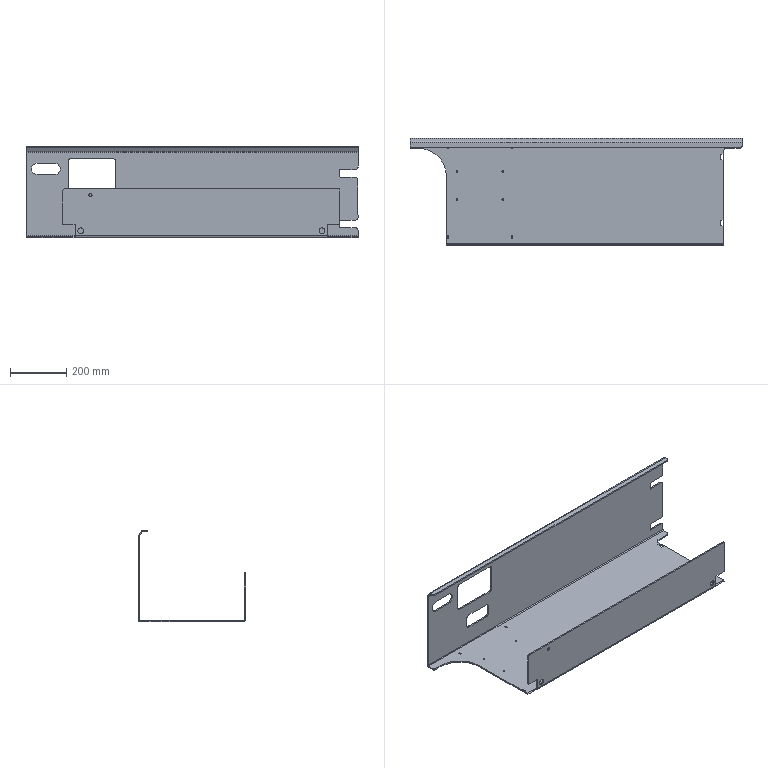Part | SolidWorks | features SM3dBend 3, Extrusion 1, FlatPattern 1, SheetMetal 1, SolidToSheetMetal 1 | 1 solid | 132 faces | box 1184 x 382 x 327.509 mm | volume 4582934 mm3 | plane 84 | cylinder 48 | commonest cylinder face diameters 20 x15 5 x8 16 x8 4 x4 6 x4 10 x3